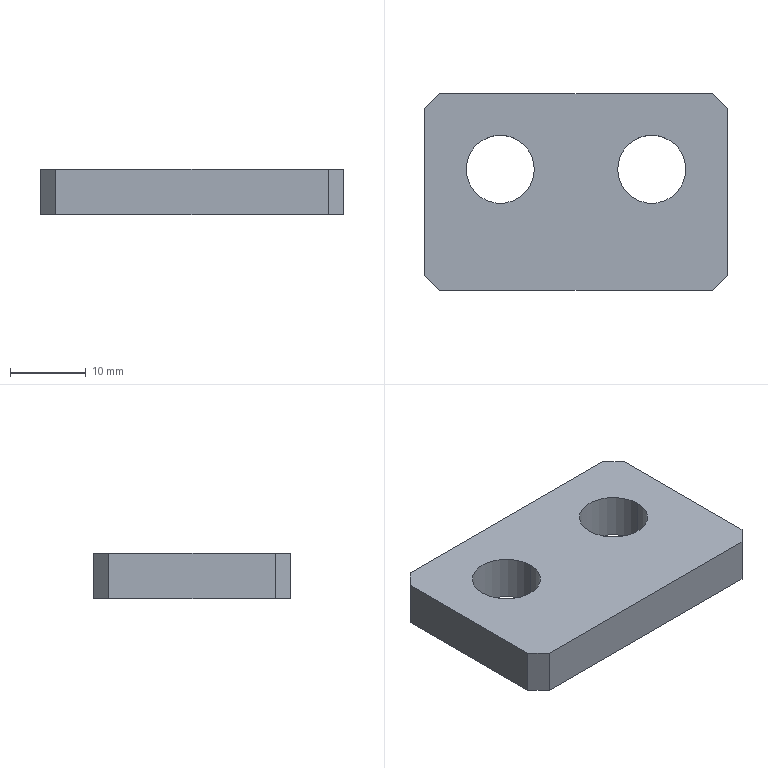Part | STEP file | 1 solid | 14 faces | box 40 x 26 x 6 mm | volume 5429 mm3 | plane 10 | cylinder 4 | commonest cylinder face diameters 9 x4
STEP:
#1=CARTESIAN_POINT('',(0.,0.,0.));
#2=DIRECTION('',(0.,0.,1.));
#3=DIRECTION('',(1.,0.,0.));
#4=AXIS2_PLACEMENT_3D('',#1,#2,#3);
#5=CARTESIAN_POINT('',(14.5,3.,6.));
#6=VERTEX_POINT('',#5);
#7=CARTESIAN_POINT('',(5.5,3.,6.));
#8=VERTEX_POINT('',#7);
#9=CARTESIAN_POINT('',(10.,3.,6.));
#10=DIRECTION('',(0.,0.,-1.));
#11=DIRECTION('',(1.,0.,0.));
#12=AXIS2_PLACEMENT_3D('',#9,#10,#11);
#13=CIRCLE('',#12,4.5);
#14=CARTESIAN_POINT('',(0.,0.,6.));
#15=DIRECTION('',(0.,0.,1.));
#16=DIRECTION('',(1.,0.,0.));
#17=AXIS2_PLACEMENT_3D('',#14,#15,#16);
#18=PLANE('',#17);
#19=CARTESIAN_POINT('',(14.5,3.));
#20=CARTESIAN_POINT('',(14.5,-4.794));
#21=CARTESIAN_POINT('',(7.75,-0.8971));
#22=CARTESIAN_POINT('',(1.,3.));
#23=CARTESIAN_POINT('',(7.75,6.897));
#24=CARTESIAN_POINT('',(14.5,10.794));
#25=CARTESIAN_POINT('',(14.5,3.));
#26=(BOUNDED_CURVE()B_SPLINE_CURVE(2,(#19,#20,#21,#22,#23,#24,#25),.UNSPECIFIED.,.T.,.F.)B_SPLINE_CURVE_WITH_KNOTS((1,2,2,2,2,1),(-2.094,0.,2.094,4.189,6.283,8.378),.UNSPECIFIED.)CURVE()GEOMETRIC_REPRESENTATION_ITEM()RATIONAL_B_SPLINE_CURVE((1.,0.5,1.,0.5,1.,0.5,1.))REPRESENTATION_ITEM(''));
#27=(GEOMETRIC_REPRESENTATION_CONTEXT(2)PARAMETRIC_REPRESENTATION_CONTEXT()REPRESENTATION_CONTEXT('',''));
#28=DEFINITIONAL_REPRESENTATION('',(#26),#27);
#29=PCURVE('',#18,#28);
#30=CARTESIAN_POINT('',(10.,3.,-0.001));
#31=DIRECTION('',(0.,0.,1.));
#32=DIRECTION('',(1.,0.,0.));
#33=AXIS2_PLACEMENT_3D('',#30,#31,#32);
#34=CYLINDRICAL_SURFACE('',#33,4.5);
#35=CARTESIAN_POINT('',(6.283,6.001));
#36=DIRECTION('',(-1.,0.));
#37=VECTOR('',#36,1.);
#38=LINE('',#35,#37);
#39=(GEOMETRIC_REPRESENTATION_CONTEXT(2)PARAMETRIC_REPRESENTATION_CONTEXT()REPRESENTATION_CONTEXT('',''));
#40=DEFINITIONAL_REPRESENTATION('',(#38),#39);
#41=PCURVE('',#34,#40);
#42=SURFACE_CURVE('',#13,(#29,#41),.PCURVE_S1.);
#43=EDGE_CURVE('',#6,#8,#42,.T.);
#44=ORIENTED_EDGE('',*,*,#43,.T.);
#45=CARTESIAN_POINT('',(10.,3.,6.));
#46=DIRECTION('',(0.,0.,-1.));
#47=DIRECTION('',(1.,0.,0.));
#48=AXIS2_PLACEMENT_3D('',#45,#46,#47);
#49=CIRCLE('',#48,4.5);
#50=CARTESIAN_POINT('',(14.5,3.));
#51=CARTESIAN_POINT('',(14.5,-4.794));
#52=CARTESIAN_POINT('',(7.75,-0.8971));
#53=CARTESIAN_POINT('',(1.,3.));
#54=CARTESIAN_POINT('',(7.75,6.897));
#55=CARTESIAN_POINT('',(14.5,10.794));
#56=CARTESIAN_POINT('',(14.5,3.));
#57=(BOUNDED_CURVE()B_SPLINE_CURVE(2,(#50,#51,#52,#53,#54,#55,#56),.UNSPECIFIED.,.T.,.F.)B_SPLINE_CURVE_WITH_KNOTS((1,2,2,2,2,1),(-2.094,0.,2.094,4.189,6.283,8.378),.UNSPECIFIED.)CURVE()GEOMETRIC_REPRESENTATION_ITEM()RATIONAL_B_SPLINE_CURVE((1.,0.5,1.,0.5,1.,0.5,1.))REPRESENTATION_ITEM(''));
#58=(GEOMETRIC_REPRESENTATION_CONTEXT(2)PARAMETRIC_REPRESENTATION_CONTEXT()REPRESENTATION_CONTEXT('',''));
#59=DEFINITIONAL_REPRESENTATION('',(#57),#58);
#60=PCURVE('',#18,#59);
#61=CARTESIAN_POINT('',(10.,3.,-0.001));
#62=DIRECTION('',(0.,0.,1.));
#63=DIRECTION('',(1.,0.,0.));
#64=AXIS2_PLACEMENT_3D('',#61,#62,#63);
#65=CYLINDRICAL_SURFACE('',#64,4.5);
#66=CARTESIAN_POINT('',(6.283,6.001));
#67=DIRECTION('',(-1.,0.));
#68=VECTOR('',#67,1.);
#69=LINE('',#66,#68);
#70=(GEOMETRIC_REPRESENTATION_CONTEXT(2)PARAMETRIC_REPRESENTATION_CONTEXT()REPRESENTATION_CONTEXT('',''));
#71=DEFINITIONAL_REPRESENTATION('',(#69),#70);
#72=PCURVE('',#65,#71);
#73=SURFACE_CURVE('',#49,(#60,#72),.PCURVE_S1.);
#74=EDGE_CURVE('',#8,#6,#73,.T.);
#75=ORIENTED_EDGE('',*,*,#74,.T.);
#76=EDGE_LOOP('',(#44,#75));
#77=FACE_BOUND('',#76,.T.);
#78=CARTESIAN_POINT('',(-5.5,3.,6.));
#79=VERTEX_POINT('',#78);
#80=CARTESIAN_POINT('',(-14.5,3.,6.));
#81=VERTEX_POINT('',#80);
#82=CARTESIAN_POINT('',(-10.,3.,6.));
#83=DIRECTION('',(0.,0.,-1.));
#84=DIRECTION('',(1.,0.,0.));
#85=AXIS2_PLACEMENT_3D('',#82,#83,#84);
#86=CIRCLE('',#85,4.5);
#87=CARTESIAN_POINT('',(-5.5,3.));
#88=CARTESIAN_POINT('',(-5.5,-4.794));
#89=CARTESIAN_POINT('',(-12.25,-0.8971));
#90=CARTESIAN_POINT('',(-19.,3.));
#91=CARTESIAN_POINT('',(-12.25,6.897));
#92=CARTESIAN_POINT('',(-5.5,10.794));
#93=CARTESIAN_POINT('',(-5.5,3.));
#94=(BOUNDED_CURVE()B_SPLINE_CURVE(2,(#87,#88,#89,#90,#91,#92,#93),.UNSPECIFIED.,.T.,.F.)B_SPLINE_CURVE_WITH_KNOTS((1,2,2,2,2,1),(-2.094,0.,2.094,4.189,6.283,8.378),.UNSPECIFIED.)CURVE()GEOMETRIC_REPRESENTATION_ITEM()RATIONAL_B_SPLINE_CURVE((1.,0.5,1.,0.5,1.,0.5,1.))REPRESENTATION_ITEM(''));
#95=(GEOMETRIC_REPRESENTATION_CONTEXT(2)PARAMETRIC_REPRESENTATION_CONTEXT()REPRESENTATION_CONTEXT('',''));
#96=DEFINITIONAL_REPRESENTATION('',(#94),#95);
#97=PCURVE('',#18,#96);
#98=CARTESIAN_POINT('',(-10.,3.,-0.001));
#99=DIRECTION('',(0.,0.,1.));
#100=DIRECTION('',(1.,0.,0.));
#101=AXIS2_PLACEMENT_3D('',#98,#99,#100);
#102=CYLINDRICAL_SURFACE('',#101,4.5);
#103=CARTESIAN_POINT('',(6.283,6.001));
#104=DIRECTION('',(-1.,0.));
#105=VECTOR('',#104,1.);
#106=LINE('',#103,#105);
#107=(GEOMETRIC_REPRESENTATION_CONTEXT(2)PARAMETRIC_REPRESENTATION_CONTEXT()REPRESENTATION_CONTEXT('',''));
#108=DEFINITIONAL_REPRESENTATION('',(#106),#107);
#109=PCURVE('',#102,#108);
#110=SURFACE_CURVE('',#86,(#97,#109),.PCURVE_S1.);
#111=EDGE_CURVE('',#79,#81,#110,.T.);
#112=ORIENTED_EDGE('',*,*,#111,.T.);
#113=CARTESIAN_POINT('',(-10.,3.,6.));
#114=DIRECTION('',(0.,0.,-1.));
#115=DIRECTION('',(1.,0.,0.));
#116=AXIS2_PLACEMENT_3D('',#113,#114,#115);
#117=CIRCLE('',#116,4.5);
#118=CARTESIAN_POINT('',(-5.5,3.));
#119=CARTESIAN_POINT('',(-5.5,-4.794));
#120=CARTESIAN_POINT('',(-12.25,-0.8971));
#121=CARTESIAN_POINT('',(-19.,3.));
#122=CARTESIAN_POINT('',(-12.25,6.897));
#123=CARTESIAN_POINT('',(-5.5,10.794));
#124=CARTESIAN_POINT('',(-5.5,3.));
#125=(BOUNDED_CURVE()B_SPLINE_CURVE(2,(#118,#119,#120,#121,#122,#123,#124),.UNSPECIFIED.,.T.,.F.)B_SPLINE_CURVE_WITH_KNOTS((1,2,2,2,2,1),(-2.094,0.,2.094,4.189,6.283,8.378),.UNSPECIFIED.)CURVE()GEOMETRIC_REPRESENTATION_ITEM()RATIONAL_B_SPLINE_CURVE((1.,0.5,1.,0.5,1.,0.5,1.))REPRESENTATION_ITEM(''));
#126=(GEOMETRIC_REPRESENTATION_CONTEXT(2)PARAMETRIC_REPRESENTATION_CONTEXT()REPRESENTATION_CONTEXT('',''));
#127=DEFINITIONAL_REPRESENTATION('',(#125),#126);
#128=PCURVE('',#18,#127);
#129=CARTESIAN_POINT('',(-10.,3.,-0.001));
#130=DIRECTION('',(0.,0.,1.));
#131=DIRECTION('',(1.,0.,0.));
#132=AXIS2_PLACEMENT_3D('',#129,#130,#131);
#133=CYLINDRICAL_SURFACE('',#132,4.5);
#134=CARTESIAN_POINT('',(6.283,6.001));
#135=DIRECTION('',(-1.,0.));
#136=VECTOR('',#135,1.);
#137=LINE('',#134,#136);
#138=(GEOMETRIC_REPRESENTATION_CONTEXT(2)PARAMETRIC_REPRESENTATION_CONTEXT()REPRESENTATION_CONTEXT('',''));
#139=DEFINITIONAL_REPRESENTATION('',(#137),#138);
#140=PCURVE('',#133,#139);
#141=SURFACE_CURVE('',#117,(#128,#140),.PCURVE_S1.);
#142=EDGE_CURVE('',#81,#79,#141,.T.);
#143=ORIENTED_EDGE('',*,*,#142,.T.);
#144=EDGE_LOOP('',(#112,#143));
#145=FACE_BOUND('',#144,.T.);
#146=CARTESIAN_POINT('',(18.,13.,6.));
#147=VERTEX_POINT('',#146);
#148=CARTESIAN_POINT('',(-18.,13.,6.));
#149=VERTEX_POINT('',#148);
#150=CARTESIAN_POINT('',(20.,13.,6.));
#151=DIRECTION('',(-1.,0.,0.));
#152=VECTOR('',#151,1.);
#153=LINE('',#150,#152);
#154=CARTESIAN_POINT('',(20.,13.));
#155=DIRECTION('',(-1.,0.));
#156=VECTOR('',#155,1.);
#157=LINE('',#154,#156);
#158=(GEOMETRIC_REPRESENTATION_CONTEXT(2)PARAMETRIC_REPRESENTATION_CONTEXT()REPRESENTATION_CONTEXT('',''));
#159=DEFINITIONAL_REPRESENTATION('',(#157),#158);
#160=PCURVE('',#18,#159);
#161=CARTESIAN_POINT('',(20.,13.,6.));
#162=DIRECTION('',(0.,-1.,0.));
#163=DIRECTION('',(0.,0.,-1.));
#164=AXIS2_PLACEMENT_3D('',#161,#162,#163);
#165=PLANE('',#164);
#166=CARTESIAN_POINT('',(0.,0.));
#167=DIRECTION('',(0.,-1.));
#168=VECTOR('',#167,1.);
#169=LINE('',#166,#168);
#170=(GEOMETRIC_REPRESENTATION_CONTEXT(2)PARAMETRIC_REPRESENTATION_CONTEXT()REPRESENTATION_CONTEXT('',''));
#171=DEFINITIONAL_REPRESENTATION('',(#169),#170);
#172=PCURVE('',#165,#171);
#173=SURFACE_CURVE('',#153,(#160,#172),.PCURVE_S1.);
#174=EDGE_CURVE('',#147,#149,#173,.T.);
#175=ORIENTED_EDGE('',*,*,#174,.T.);
#176=CARTESIAN_POINT('',(-20.,11.,6.));
#177=VERTEX_POINT('',#176);
#178=CARTESIAN_POINT('',(-20.,11.,6.));
#179=DIRECTION('',(-0.7071,-0.7071,0.));
#180=VECTOR('',#179,1.);
#181=LINE('',#178,#180);
#182=CARTESIAN_POINT('',(-20.,11.));
#183=DIRECTION('',(-0.7071,-0.7071));
#184=VECTOR('',#183,1.);
#185=LINE('',#182,#184);
#186=(GEOMETRIC_REPRESENTATION_CONTEXT(2)PARAMETRIC_REPRESENTATION_CONTEXT()REPRESENTATION_CONTEXT('',''));
#187=DEFINITIONAL_REPRESENTATION('',(#185),#186);
#188=PCURVE('',#18,#187);
#189=CARTESIAN_POINT('',(-20.,11.,6.));
#190=DIRECTION('',(0.7071,-0.7071,0.));
#191=DIRECTION('',(0.,0.,-1.));
#192=AXIS2_PLACEMENT_3D('',#189,#190,#191);
#193=PLANE('',#192);
#194=CARTESIAN_POINT('',(0.,0.));
#195=DIRECTION('',(0.,-1.));
#196=VECTOR('',#195,1.);
#197=LINE('',#194,#196);
#198=(GEOMETRIC_REPRESENTATION_CONTEXT(2)PARAMETRIC_REPRESENTATION_CONTEXT()REPRESENTATION_CONTEXT('',''));
#199=DEFINITIONAL_REPRESENTATION('',(#197),#198);
#200=PCURVE('',#193,#199);
#201=SURFACE_CURVE('',#181,(#188,#200),.PCURVE_S1.);
#202=EDGE_CURVE('',#149,#177,#201,.T.);
#203=ORIENTED_EDGE('',*,*,#202,.T.);
#204=CARTESIAN_POINT('',(-20.,-11.,6.));
#205=VERTEX_POINT('',#204);
#206=CARTESIAN_POINT('',(-20.,-13.,6.));
#207=DIRECTION('',(0.,-1.,0.));
#208=VECTOR('',#207,1.);
#209=LINE('',#206,#208);
#210=CARTESIAN_POINT('',(-20.,-13.));
#211=DIRECTION('',(0.,-1.));
#212=VECTOR('',#211,1.);
#213=LINE('',#210,#212);
#214=(GEOMETRIC_REPRESENTATION_CONTEXT(2)PARAMETRIC_REPRESENTATION_CONTEXT()REPRESENTATION_CONTEXT('',''));
#215=DEFINITIONAL_REPRESENTATION('',(#213),#214);
#216=PCURVE('',#18,#215);
#217=CARTESIAN_POINT('',(-20.,-13.,6.));
#218=DIRECTION('',(1.,0.,0.));
#219=DIRECTION('',(0.,1.,0.));
#220=AXIS2_PLACEMENT_3D('',#217,#218,#219);
#221=PLANE('',#220);
#222=CARTESIAN_POINT('',(0.,0.));
#223=DIRECTION('',(-1.,0.));
#224=VECTOR('',#223,1.);
#225=LINE('',#222,#224);
#226=(GEOMETRIC_REPRESENTATION_CONTEXT(2)PARAMETRIC_REPRESENTATION_CONTEXT()REPRESENTATION_CONTEXT('',''));
#227=DEFINITIONAL_REPRESENTATION('',(#225),#226);
#228=PCURVE('',#221,#227);
#229=SURFACE_CURVE('',#209,(#216,#228),.PCURVE_S1.);
#230=EDGE_CURVE('',#177,#205,#229,.T.);
#231=ORIENTED_EDGE('',*,*,#230,.T.);
#232=CARTESIAN_POINT('',(-18.,-13.,6.));
#233=VERTEX_POINT('',#232);
#234=CARTESIAN_POINT('',(-18.,-13.,6.));
#235=DIRECTION('',(0.7071,-0.7071,0.));
#236=VECTOR('',#235,1.);
#237=LINE('',#234,#236);
#238=CARTESIAN_POINT('',(-18.,-13.));
#239=DIRECTION('',(0.7071,-0.7071));
#240=VECTOR('',#239,1.);
#241=LINE('',#238,#240);
#242=(GEOMETRIC_REPRESENTATION_CONTEXT(2)PARAMETRIC_REPRESENTATION_CONTEXT()REPRESENTATION_CONTEXT('',''));
#243=DEFINITIONAL_REPRESENTATION('',(#241),#242);
#244=PCURVE('',#18,#243);
#245=CARTESIAN_POINT('',(-18.,-13.,6.));
#246=DIRECTION('',(0.7071,0.7071,0.));
#247=DIRECTION('',(0.,0.,-1.));
#248=AXIS2_PLACEMENT_3D('',#245,#246,#247);
#249=PLANE('',#248);
#250=CARTESIAN_POINT('',(0.,0.));
#251=DIRECTION('',(0.,-1.));
#252=VECTOR('',#251,1.);
#253=LINE('',#250,#252);
#254=(GEOMETRIC_REPRESENTATION_CONTEXT(2)PARAMETRIC_REPRESENTATION_CONTEXT()REPRESENTATION_CONTEXT('',''));
#255=DEFINITIONAL_REPRESENTATION('',(#253),#254);
#256=PCURVE('',#249,#255);
#257=SURFACE_CURVE('',#237,(#244,#256),.PCURVE_S1.);
#258=EDGE_CURVE('',#205,#233,#257,.T.);
#259=ORIENTED_EDGE('',*,*,#258,.T.);
#260=CARTESIAN_POINT('',(18.,-13.,6.));
#261=VERTEX_POINT('',#260);
#262=CARTESIAN_POINT('',(20.,-13.,6.));
#263=DIRECTION('',(1.,0.,0.));
#264=VECTOR('',#263,1.);
#265=LINE('',#262,#264);
#266=CARTESIAN_POINT('',(20.,-13.));
#267=DIRECTION('',(1.,0.));
#268=VECTOR('',#267,1.);
#269=LINE('',#266,#268);
#270=(GEOMETRIC_REPRESENTATION_CONTEXT(2)PARAMETRIC_REPRESENTATION_CONTEXT()REPRESENTATION_CONTEXT('',''));
#271=DEFINITIONAL_REPRESENTATION('',(#269),#270);
#272=PCURVE('',#18,#271);
#273=CARTESIAN_POINT('',(20.,-13.,6.));
#274=DIRECTION('',(0.,1.,0.));
#275=DIRECTION('',(1.,0.,0.));
#276=AXIS2_PLACEMENT_3D('',#273,#274,#275);
#277=PLANE('',#276);
#278=CARTESIAN_POINT('',(0.,0.));
#279=DIRECTION('',(1.,0.));
#280=VECTOR('',#279,1.);
#281=LINE('',#278,#280);
#282=(GEOMETRIC_REPRESENTATION_CONTEXT(2)PARAMETRIC_REPRESENTATION_CONTEXT()REPRESENTATION_CONTEXT('',''));
#283=DEFINITIONAL_REPRESENTATION('',(#281),#282);
#284=PCURVE('',#277,#283);
#285=SURFACE_CURVE('',#265,(#272,#284),.PCURVE_S1.);
#286=EDGE_CURVE('',#233,#261,#285,.T.);
#287=ORIENTED_EDGE('',*,*,#286,.T.);
#288=CARTESIAN_POINT('',(20.,-11.,6.));
#289=VERTEX_POINT('',#288);
#290=CARTESIAN_POINT('',(20.,-11.,6.));
#291=DIRECTION('',(0.7071,0.7071,0.));
#292=VECTOR('',#291,1.);
#293=LINE('',#290,#292);
#294=CARTESIAN_POINT('',(20.,-11.));
#295=DIRECTION('',(0.7071,0.7071));
#296=VECTOR('',#295,1.);
#297=LINE('',#294,#296);
#298=(GEOMETRIC_REPRESENTATION_CONTEXT(2)PARAMETRIC_REPRESENTATION_CONTEXT()REPRESENTATION_CONTEXT('',''));
#299=DEFINITIONAL_REPRESENTATION('',(#297),#298);
#300=PCURVE('',#18,#299);
#301=CARTESIAN_POINT('',(20.,-11.,6.));
#302=DIRECTION('',(-0.7071,0.7071,0.));
#303=DIRECTION('',(0.,0.,1.));
#304=AXIS2_PLACEMENT_3D('',#301,#302,#303);
#305=PLANE('',#304);
#306=CARTESIAN_POINT('',(0.,0.));
#307=DIRECTION('',(0.,1.));
#308=VECTOR('',#307,1.);
#309=LINE('',#306,#308);
#310=(GEOMETRIC_REPRESENTATION_CONTEXT(2)PARAMETRIC_REPRESENTATION_CONTEXT()REPRESENTATION_CONTEXT('',''));
#311=DEFINITIONAL_REPRESENTATION('',(#309),#310);
#312=PCURVE('',#305,#311);
#313=SURFACE_CURVE('',#293,(#300,#312),.PCURVE_S1.);
#314=EDGE_CURVE('',#261,#289,#313,.T.);
#315=ORIENTED_EDGE('',*,*,#314,.T.);
#316=CARTESIAN_POINT('',(20.,11.,6.));
#317=VERTEX_POINT('',#316);
#318=CARTESIAN_POINT('',(20.,-13.,6.));
#319=DIRECTION('',(0.,1.,0.));
#320=VECTOR('',#319,1.);
#321=LINE('',#318,#320);
#322=CARTESIAN_POINT('',(20.,-13.));
#323=DIRECTION('',(0.,1.));
#324=VECTOR('',#323,1.);
#325=LINE('',#322,#324);
#326=(GEOMETRIC_REPRESENTATION_CONTEXT(2)PARAMETRIC_REPRESENTATION_CONTEXT()REPRESENTATION_CONTEXT('',''));
#327=DEFINITIONAL_REPRESENTATION('',(#325),#326);
#328=PCURVE('',#18,#327);
#329=CARTESIAN_POINT('',(20.,-13.,6.));
#330=DIRECTION('',(-1.,0.,0.));
#331=DIRECTION('',(0.,0.,1.));
#332=AXIS2_PLACEMENT_3D('',#329,#330,#331);
#333=PLANE('',#332);
#334=CARTESIAN_POINT('',(0.,0.));
#335=DIRECTION('',(0.,1.));
#336=VECTOR('',#335,1.);
#337=LINE('',#334,#336);
#338=(GEOMETRIC_REPRESENTATION_CONTEXT(2)PARAMETRIC_REPRESENTATION_CONTEXT()REPRESENTATION_CONTEXT('',''));
#339=DEFINITIONAL_REPRESENTATION('',(#337),#338);
#340=PCURVE('',#333,#339);
#341=SURFACE_CURVE('',#321,(#328,#340),.PCURVE_S1.);
#342=EDGE_CURVE('',#289,#317,#341,.T.);
#343=ORIENTED_EDGE('',*,*,#342,.T.);
#344=CARTESIAN_POINT('',(18.,13.,6.));
#345=DIRECTION('',(-0.7071,0.7071,0.));
#346=VECTOR('',#345,1.);
#347=LINE('',#344,#346);
#348=CARTESIAN_POINT('',(18.,13.));
#349=DIRECTION('',(-0.7071,0.7071));
#350=VECTOR('',#349,1.);
#351=LINE('',#348,#350);
#352=(GEOMETRIC_REPRESENTATION_CONTEXT(2)PARAMETRIC_REPRESENTATION_CONTEXT()REPRESENTATION_CONTEXT('',''));
#353=DEFINITIONAL_REPRESENTATION('',(#351),#352);
#354=PCURVE('',#18,#353);
#355=CARTESIAN_POINT('',(18.,13.,6.));
#356=DIRECTION('',(-0.7071,-0.7071,0.));
#357=DIRECTION('',(-0.7071,0.7071,0.));
#358=AXIS2_PLACEMENT_3D('',#355,#356,#357);
#359=PLANE('',#358);
#360=CARTESIAN_POINT('',(0.,0.));
#361=DIRECTION('',(1.,0.));
#362=VECTOR('',#361,1.);
#363=LINE('',#360,#362);
#364=(GEOMETRIC_REPRESENTATION_CONTEXT(2)PARAMETRIC_REPRESENTATION_CONTEXT()REPRESENTATION_CONTEXT('',''));
#365=DEFINITIONAL_REPRESENTATION('',(#363),#364);
#366=PCURVE('',#359,#365);
#367=SURFACE_CURVE('',#347,(#354,#366),.PCURVE_S1.);
#368=EDGE_CURVE('',#317,#147,#367,.T.);
#369=ORIENTED_EDGE('',*,*,#368,.T.);
#370=EDGE_LOOP('',(#175,#203,#231,#259,#287,#315,#343,#369));
#371=FACE_BOUND('',#370,.T.);
#372=ADVANCED_FACE('',(#77,#145,#371),#18,.T.);
#373=ORIENTED_EDGE('',*,*,#74,.T.);
#374=CARTESIAN_POINT('',(14.5,3.,0.));
#375=VERTEX_POINT('',#374);
#376=CARTESIAN_POINT('',(14.5,3.,-0.001));
#377=DIRECTION('',(0.,0.,1.));
#378=VECTOR('',#377,1.);
#379=LINE('',#376,#378);
#380=CARTESIAN_POINT('',(0.,0.));
#381=DIRECTION('',(0.,1.));
#382=VECTOR('',#381,1.);
#383=LINE('',#380,#382);
#384=(GEOMETRIC_REPRESENTATION_CONTEXT(2)PARAMETRIC_REPRESENTATION_CONTEXT()REPRESENTATION_CONTEXT('',''));
#385=DEFINITIONAL_REPRESENTATION('',(#383),#384);
#386=PCURVE('',#65,#385);
#387=CARTESIAN_POINT('',(6.283,0.));
#388=DIRECTION('',(0.,1.));
#389=VECTOR('',#388,1.);
#390=LINE('',#387,#389);
#391=(GEOMETRIC_REPRESENTATION_CONTEXT(2)PARAMETRIC_REPRESENTATION_CONTEXT()REPRESENTATION_CONTEXT('',''));
#392=DEFINITIONAL_REPRESENTATION('',(#390),#391);
#393=PCURVE('',#34,#392);
#394=SURFACE_CURVE('',#379,(#386,#393),.PCURVE_S1.);
#395=EDGE_CURVE('',#375,#6,#394,.T.);
#396=ORIENTED_EDGE('',*,*,#395,.F.);
#397=CARTESIAN_POINT('',(5.5,3.,0.));
#398=VERTEX_POINT('',#397);
#399=CARTESIAN_POINT('',(10.,3.,0.));
#400=DIRECTION('',(0.,0.,-1.));
#401=DIRECTION('',(1.,0.,0.));
#402=AXIS2_PLACEMENT_3D('',#399,#400,#401);
#403=CIRCLE('',#402,4.5);
#404=CARTESIAN_POINT('',(6.283,0.001));
#405=DIRECTION('',(-1.,0.));
#406=VECTOR('',#405,1.);
#407=LINE('',#404,#406);
#408=(GEOMETRIC_REPRESENTATION_CONTEXT(2)PARAMETRIC_REPRESENTATION_CONTEXT()REPRESENTATION_CONTEXT('',''));
#409=DEFINITIONAL_REPRESENTATION('',(#407),#408);
#410=PCURVE('',#65,#409);
#411=CARTESIAN_POINT('',(0.,0.,0.));
#412=DIRECTION('',(0.,0.,1.));
#413=DIRECTION('',(1.,0.,0.));
#414=AXIS2_PLACEMENT_3D('',#411,#412,#413);
#415=PLANE('',#414);
#416=CARTESIAN_POINT('',(14.5,3.));
#417=CARTESIAN_POINT('',(14.5,-4.794));
#418=CARTESIAN_POINT('',(7.75,-0.8971));
#419=CARTESIAN_POINT('',(1.,3.));
#420=CARTESIAN_POINT('',(7.75,6.897));
#421=CARTESIAN_POINT('',(14.5,10.794));
#422=CARTESIAN_POINT('',(14.5,3.));
#423=(BOUNDED_CURVE()B_SPLINE_CURVE(2,(#416,#417,#418,#419,#420,#421,#422),.UNSPECIFIED.,.T.,.F.)B_SPLINE_CURVE_WITH_KNOTS((1,2,2,2,2,1),(-2.094,0.,2.094,4.189,6.283,8.378),.UNSPECIFIED.)CURVE()GEOMETRIC_REPRESENTATION_ITEM()RATIONAL_B_SPLINE_CURVE((1.,0.5,1.,0.5,1.,0.5,1.))REPRESENTATION_ITEM(''));
#424=(GEOMETRIC_REPRESENTATION_CONTEXT(2)PARAMETRIC_REPRESENTATION_CONTEXT()REPRESENTATION_CONTEXT('',''));
#425=DEFINITIONAL_REPRESENTATION('',(#423),#424);
#426=PCURVE('',#415,#425);
#427=SURFACE_CURVE('',#403,(#410,#426),.PCURVE_S1.);
#428=EDGE_CURVE('',#398,#375,#427,.T.);
#429=ORIENTED_EDGE('',*,*,#428,.F.);
#430=CARTESIAN_POINT('',(5.5,3.,-0.001));
#431=DIRECTION('',(0.,0.,1.));
#432=VECTOR('',#431,1.);
#433=LINE('',#430,#432);
#434=CARTESIAN_POINT('',(3.142,0.));
#435=DIRECTION('',(0.,1.));
#436=VECTOR('',#435,1.);
#437=LINE('',#434,#436);
#438=(GEOMETRIC_REPRESENTATION_CONTEXT(2)PARAMETRIC_REPRESENTATION_CONTEXT()REPRESENTATION_CONTEXT('',''));
#439=DEFINITIONAL_REPRESENTATION('',(#437),#438);
#440=PCURVE('',#65,#439);
#441=CARTESIAN_POINT('',(3.142,0.));
#442=DIRECTION('',(0.,1.));
#443=VECTOR('',#442,1.);
#444=LINE('',#441,#443);
#445=(GEOMETRIC_REPRESENTATION_CONTEXT(2)PARAMETRIC_REPRESENTATION_CONTEXT()REPRESENTATION_CONTEXT('',''));
#446=DEFINITIONAL_REPRESENTATION('',(#444),#445);
#447=PCURVE('',#34,#446);
#448=SURFACE_CURVE('',#433,(#440,#447),.PCURVE_S1.);
#449=EDGE_CURVE('',#398,#8,#448,.T.);
#450=ORIENTED_EDGE('',*,*,#449,.T.);
#451=EDGE_LOOP('',(#373,#396,#429,#450));
#452=FACE_BOUND('',#451,.F.);
#453=ADVANCED_FACE('',(#452),#65,.F.);
#454=ORIENTED_EDGE('',*,*,#142,.T.);
#455=CARTESIAN_POINT('',(-5.5,3.,0.));
#456=VERTEX_POINT('',#455);
#457=CARTESIAN_POINT('',(-5.5,3.,-0.001));
#458=DIRECTION('',(0.,0.,1.));
#459=VECTOR('',#458,1.);
#460=LINE('',#457,#459);
#461=CARTESIAN_POINT('',(0.,0.));
#462=DIRECTION('',(0.,1.));
#463=VECTOR('',#462,1.);
#464=LINE('',#461,#463);
#465=(GEOMETRIC_REPRESENTATION_CONTEXT(2)PARAMETRIC_REPRESENTATION_CONTEXT()REPRESENTATION_CONTEXT('',''));
#466=DEFINITIONAL_REPRESENTATION('',(#464),#465);
#467=PCURVE('',#133,#466);
#468=CARTESIAN_POINT('',(6.283,0.));
#469=DIRECTION('',(0.,1.));
#470=VECTOR('',#469,1.);
#471=LINE('',#468,#470);
#472=(GEOMETRIC_REPRESENTATION_CONTEXT(2)PARAMETRIC_REPRESENTATION_CONTEXT()REPRESENTATION_CONTEXT('',''));
#473=DEFINITIONAL_REPRESENTATION('',(#471),#472);
#474=PCURVE('',#102,#473);
#475=SURFACE_CURVE('',#460,(#467,#474),.PCURVE_S1.);
#476=EDGE_CURVE('',#456,#79,#475,.T.);
#477=ORIENTED_EDGE('',*,*,#476,.F.);
#478=CARTESIAN_POINT('',(-14.5,3.,0.));
#479=VERTEX_POINT('',#478);
#480=CARTESIAN_POINT('',(-10.,3.,0.));
#481=DIRECTION('',(0.,0.,-1.));
#482=DIRECTION('',(1.,0.,0.));
#483=AXIS2_PLACEMENT_3D('',#480,#481,#482);
#484=CIRCLE('',#483,4.5);
#485=CARTESIAN_POINT('',(6.283,0.001));
#486=DIRECTION('',(-1.,0.));
#487=VECTOR('',#486,1.);
#488=LINE('',#485,#487);
#489=(GEOMETRIC_REPRESENTATION_CONTEXT(2)PARAMETRIC_REPRESENTATION_CONTEXT()REPRESENTATION_CONTEXT('',''));
#490=DEFINITIONAL_REPRESENTATION('',(#488),#489);
#491=PCURVE('',#133,#490);
#492=CARTESIAN_POINT('',(-5.5,3.));
#493=CARTESIAN_POINT('',(-5.5,-4.794));
#494=CARTESIAN_POINT('',(-12.25,-0.8971));
#495=CARTESIAN_POINT('',(-19.,3.));
#496=CARTESIAN_POINT('',(-12.25,6.897));
#497=CARTESIAN_POINT('',(-5.5,10.794));
#498=CARTESIAN_POINT('',(-5.5,3.));
#499=(BOUNDED_CURVE()B_SPLINE_CURVE(2,(#492,#493,#494,#495,#496,#497,#498),.UNSPECIFIED.,.T.,.F.)B_SPLINE_CURVE_WITH_KNOTS((1,2,2,2,2,1),(-2.094,0.,2.094,4.189,6.283,8.378),.UNSPECIFIED.)CURVE()GEOMETRIC_REPRESENTATION_ITEM()RATIONAL_B_SPLINE_CURVE((1.,0.5,1.,0.5,1.,0.5,1.))REPRESENTATION_ITEM(''));
#500=(GEOMETRIC_REPRESENTATION_CONTEXT(2)PARAMETRIC_REPRESENTATION_CONTEXT()REPRESENTATION_CONTEXT('',''));
#501=DEFINITIONAL_REPRESENTATION('',(#499),#500);
#502=PCURVE('',#415,#501);
#503=SURFACE_CURVE('',#484,(#491,#502),.PCURVE_S1.);
#504=EDGE_CURVE('',#479,#456,#503,.T.);
#505=ORIENTED_EDGE('',*,*,#504,.F.);
#506=CARTESIAN_POINT('',(-14.5,3.,-0.001));
#507=DIRECTION('',(0.,0.,1.));
#508=VECTOR('',#507,1.);
#509=LINE('',#506,#508);
#510=CARTESIAN_POINT('',(3.142,0.));
#511=DIRECTION('',(0.,1.));
#512=VECTOR('',#511,1.);
#513=LINE('',#510,#512);
#514=(GEOMETRIC_REPRESENTATION_CONTEXT(2)PARAMETRIC_REPRESENTATION_CONTEXT()REPRESENTATION_CONTEXT('',''));
#515=DEFINITIONAL_REPRESENTATION('',(#513),#514);
#516=PCURVE('',#133,#515);
#517=CARTESIAN_POINT('',(3.142,0.));
#518=DIRECTION('',(0.,1.));
#519=VECTOR('',#518,1.);
#520=LINE('',#517,#519);
#521=(GEOMETRIC_REPRESENTATION_CONTEXT(2)PARAMETRIC_REPRESENTATION_CONTEXT()REPRESENTATION_CONTEXT('',''));
#522=DEFINITIONAL_REPRESENTATION('',(#520),#521);
#523=PCURVE('',#102,#522);
#524=SURFACE_CURVE('',#509,(#516,#523),.PCURVE_S1.);
#525=EDGE_CURVE('',#479,#81,#524,.T.);
#526=ORIENTED_EDGE('',*,*,#525,.T.);
#527=EDGE_LOOP('',(#454,#477,#505,#526));
#528=FACE_BOUND('',#527,.F.);
#529=ADVANCED_FACE('',(#528),#133,.F.);
#530=CARTESIAN_POINT('',(18.,-13.,0.));
#531=VERTEX_POINT('',#530);
#532=CARTESIAN_POINT('',(18.,-13.,6.));
#533=DIRECTION('',(0.,0.,-1.));
#534=VECTOR('',#533,1.);
#535=LINE('',#532,#534);
#536=CARTESIAN_POINT('',(0.,-2.828));
#537=DIRECTION('',(-1.,0.));
#538=VECTOR('',#537,1.);
#539=LINE('',#536,#538);
#540=(GEOMETRIC_REPRESENTATION_CONTEXT(2)PARAMETRIC_REPRESENTATION_CONTEXT()REPRESENTATION_CONTEXT('',''));
#541=DEFINITIONAL_REPRESENTATION('',(#539),#540);
#542=PCURVE('',#305,#541);
#543=CARTESIAN_POINT('',(-2.,0.));
#544=DIRECTION('',(0.,1.));
#545=VECTOR('',#544,1.);
#546=LINE('',#543,#545);
#547=(GEOMETRIC_REPRESENTATION_CONTEXT(2)PARAMETRIC_REPRESENTATION_CONTEXT()REPRESENTATION_CONTEXT('',''));
#548=DEFINITIONAL_REPRESENTATION('',(#546),#547);
#549=PCURVE('',#277,#548);
#550=SURFACE_CURVE('',#535,(#542,#549),.PCURVE_S1.);
#551=EDGE_CURVE('',#261,#531,#550,.T.);
#552=ORIENTED_EDGE('',*,*,#551,.T.);
#553=CARTESIAN_POINT('',(20.,-11.,0.));
#554=VERTEX_POINT('',#553);
#555=CARTESIAN_POINT('',(18.,-13.,0.));
#556=DIRECTION('',(0.7071,0.7071,0.));
#557=VECTOR('',#556,1.);
#558=LINE('',#555,#557);
#559=CARTESIAN_POINT('',(-6.,-2.828));
#560=DIRECTION('',(0.,1.));
#561=VECTOR('',#560,1.);
#562=LINE('',#559,#561);
#563=(GEOMETRIC_REPRESENTATION_CONTEXT(2)PARAMETRIC_REPRESENTATION_CONTEXT()REPRESENTATION_CONTEXT('',''));
#564=DEFINITIONAL_REPRESENTATION('',(#562),#563);
#565=PCURVE('',#305,#564);
#566=CARTESIAN_POINT('',(18.,-13.));
#567=DIRECTION('',(0.7071,0.7071));
#568=VECTOR('',#567,1.);
#569=LINE('',#566,#568);
#570=(GEOMETRIC_REPRESENTATION_CONTEXT(2)PARAMETRIC_REPRESENTATION_CONTEXT()REPRESENTATION_CONTEXT('',''));
#571=DEFINITIONAL_REPRESENTATION('',(#569),#570);
#572=PCURVE('',#415,#571);
#573=SURFACE_CURVE('',#558,(#565,#572),.PCURVE_S1.);
#574=EDGE_CURVE('',#531,#554,#573,.T.);
#575=ORIENTED_EDGE('',*,*,#574,.T.);
#576=CARTESIAN_POINT('',(20.,-11.,6.));
#577=DIRECTION('',(0.,0.,1.));
#578=VECTOR('',#577,1.);
#579=LINE('',#576,#578);
#580=CARTESIAN_POINT('',(0.,0.));
#581=DIRECTION('',(1.,0.));
#582=VECTOR('',#581,1.);
#583=LINE('',#580,#582);
#584=(GEOMETRIC_REPRESENTATION_CONTEXT(2)PARAMETRIC_REPRESENTATION_CONTEXT()REPRESENTATION_CONTEXT('',''));
#585=DEFINITIONAL_REPRESENTATION('',(#583),#584);
#586=PCURVE('',#305,#585);
#587=CARTESIAN_POINT('',(0.,2.));
#588=DIRECTION('',(1.,0.));
#589=VECTOR('',#588,1.);
#590=LINE('',#587,#589);
#591=(GEOMETRIC_REPRESENTATION_CONTEXT(2)PARAMETRIC_REPRESENTATION_CONTEXT()REPRESENTATION_CONTEXT('',''));
#592=DEFINITIONAL_REPRESENTATION('',(#590),#591);
#593=PCURVE('',#333,#592);
#594=SURFACE_CURVE('',#579,(#586,#593),.PCURVE_S1.);
#595=EDGE_CURVE('',#554,#289,#594,.T.);
#596=ORIENTED_EDGE('',*,*,#595,.T.);
#597=ORIENTED_EDGE('',*,*,#314,.F.);
#598=EDGE_LOOP('',(#552,#575,#596,#597));
#599=FACE_BOUND('',#598,.T.);
#600=ADVANCED_FACE('',(#599),#305,.F.);
#601=ORIENTED_EDGE('',*,*,#595,.F.);
#602=CARTESIAN_POINT('',(20.,11.,0.));
#603=VERTEX_POINT('',#602);
#604=CARTESIAN_POINT('',(20.,0.,0.));
#605=DIRECTION('',(0.,1.,0.));
#606=VECTOR('',#605,1.);
#607=LINE('',#604,#606);
#608=CARTESIAN_POINT('',(-6.,13.));
#609=DIRECTION('',(0.,1.));
#610=VECTOR('',#609,1.);
#611=LINE('',#608,#610);
#612=(GEOMETRIC_REPRESENTATION_CONTEXT(2)PARAMETRIC_REPRESENTATION_CONTEXT()REPRESENTATION_CONTEXT('',''));
#613=DEFINITIONAL_REPRESENTATION('',(#611),#612);
#614=PCURVE('',#333,#613);
#615=CARTESIAN_POINT('',(20.,0.));
#616=DIRECTION('',(0.,1.));
#617=VECTOR('',#616,1.);
#618=LINE('',#615,#617);
#619=(GEOMETRIC_REPRESENTATION_CONTEXT(2)PARAMETRIC_REPRESENTATION_CONTEXT()REPRESENTATION_CONTEXT('',''));
#620=DEFINITIONAL_REPRESENTATION('',(#618),#619);
#621=PCURVE('',#415,#620);
#622=SURFACE_CURVE('',#607,(#614,#621),.PCURVE_S1.);
#623=EDGE_CURVE('',#554,#603,#622,.T.);
#624=ORIENTED_EDGE('',*,*,#623,.T.);
#625=CARTESIAN_POINT('',(20.,11.,6.));
#626=DIRECTION('',(0.,0.,1.));
#627=VECTOR('',#626,1.);
#628=LINE('',#625,#627);
#629=CARTESIAN_POINT('',(0.,24.));
#630=DIRECTION('',(1.,0.));
#631=VECTOR('',#630,1.);
#632=LINE('',#629,#631);
#633=(GEOMETRIC_REPRESENTATION_CONTEXT(2)PARAMETRIC_REPRESENTATION_CONTEXT()REPRESENTATION_CONTEXT('',''));
#634=DEFINITIONAL_REPRESENTATION('',(#632),#633);
#635=PCURVE('',#333,#634);
#636=CARTESIAN_POINT('',(-2.828,0.));
#637=DIRECTION('',(0.,-1.));
#638=VECTOR('',#637,1.);
#639=LINE('',#636,#638);
#640=(GEOMETRIC_REPRESENTATION_CONTEXT(2)PARAMETRIC_REPRESENTATION_CONTEXT()REPRESENTATION_CONTEXT('',''));
#641=DEFINITIONAL_REPRESENTATION('',(#639),#640);
#642=PCURVE('',#359,#641);
#643=SURFACE_CURVE('',#628,(#635,#642),.PCURVE_S1.);
#644=EDGE_CURVE('',#603,#317,#643,.T.);
#645=ORIENTED_EDGE('',*,*,#644,.T.);
#646=ORIENTED_EDGE('',*,*,#342,.F.);
#647=EDGE_LOOP('',(#601,#624,#645,#646));
#648=FACE_BOUND('',#647,.T.);
#649=ADVANCED_FACE('',(#648),#333,.F.);
#650=ORIENTED_EDGE('',*,*,#644,.F.);
#651=CARTESIAN_POINT('',(18.,13.,0.));
#652=VERTEX_POINT('',#651);
#653=CARTESIAN_POINT('',(20.,11.,0.));
#654=DIRECTION('',(-0.7071,0.7071,0.));
#655=VECTOR('',#654,1.);
#656=LINE('',#653,#655);
#657=CARTESIAN_POINT('',(-2.828,6.));
#658=DIRECTION('',(1.,0.));
#659=VECTOR('',#658,1.);
#660=LINE('',#657,#659);
#661=(GEOMETRIC_REPRESENTATION_CONTEXT(2)PARAMETRIC_REPRESENTATION_CONTEXT()REPRESENTATION_CONTEXT('',''));
#662=DEFINITIONAL_REPRESENTATION('',(#660),#661);
#663=PCURVE('',#359,#662);
#664=CARTESIAN_POINT('',(20.,11.));
#665=DIRECTION('',(-0.7071,0.7071));
#666=VECTOR('',#665,1.);
#667=LINE('',#664,#666);
#668=(GEOMETRIC_REPRESENTATION_CONTEXT(2)PARAMETRIC_REPRESENTATION_CONTEXT()REPRESENTATION_CONTEXT('',''));
#669=DEFINITIONAL_REPRESENTATION('',(#667),#668);
#670=PCURVE('',#415,#669);
#671=SURFACE_CURVE('',#656,(#663,#670),.PCURVE_S1.);
#672=EDGE_CURVE('',#603,#652,#671,.T.);
#673=ORIENTED_EDGE('',*,*,#672,.T.);
#674=CARTESIAN_POINT('',(18.,13.,6.));
#675=DIRECTION('',(0.,0.,1.));
#676=VECTOR('',#675,1.);
#677=LINE('',#674,#676);
#678=CARTESIAN_POINT('',(0.,0.));
#679=DIRECTION('',(0.,-1.));
#680=VECTOR('',#679,1.);
#681=LINE('',#678,#680);
#682=(GEOMETRIC_REPRESENTATION_CONTEXT(2)PARAMETRIC_REPRESENTATION_CONTEXT()REPRESENTATION_CONTEXT('',''));
#683=DEFINITIONAL_REPRESENTATION('',(#681),#682);
#684=PCURVE('',#359,#683);
#685=CARTESIAN_POINT('',(0.,-2.));
#686=DIRECTION('',(-1.,0.));
#687=VECTOR('',#686,1.);
#688=LINE('',#685,#687);
#689=(GEOMETRIC_REPRESENTATION_CONTEXT(2)PARAMETRIC_REPRESENTATION_CONTEXT()REPRESENTATION_CONTEXT('',''));
#690=DEFINITIONAL_REPRESENTATION('',(#688),#689);
#691=PCURVE('',#165,#690);
#692=SURFACE_CURVE('',#677,(#684,#691),.PCURVE_S1.);
#693=EDGE_CURVE('',#652,#147,#692,.T.);
#694=ORIENTED_EDGE('',*,*,#693,.T.);
#695=ORIENTED_EDGE('',*,*,#368,.F.);
#696=EDGE_LOOP('',(#650,#673,#694,#695));
#697=FACE_BOUND('',#696,.T.);
#698=ADVANCED_FACE('',(#697),#359,.F.);
#699=CARTESIAN_POINT('',(-18.,13.,0.));
#700=VERTEX_POINT('',#699);
#701=CARTESIAN_POINT('',(-18.,13.,6.));
#702=DIRECTION('',(0.,0.,1.));
#703=VECTOR('',#702,1.);
#704=LINE('',#701,#703);
#705=CARTESIAN_POINT('',(0.,-38.));
#706=DIRECTION('',(-1.,0.));
#707=VECTOR('',#706,1.);
#708=LINE('',#705,#707);
#709=(GEOMETRIC_REPRESENTATION_CONTEXT(2)PARAMETRIC_REPRESENTATION_CONTEXT()REPRESENTATION_CONTEXT('',''));
#710=DEFINITIONAL_REPRESENTATION('',(#708),#709);
#711=PCURVE('',#165,#710);
#712=CARTESIAN_POINT('',(0.,2.828));
#713=DIRECTION('',(-1.,0.));
#714=VECTOR('',#713,1.);
#715=LINE('',#712,#714);
#716=(GEOMETRIC_REPRESENTATION_CONTEXT(2)PARAMETRIC_REPRESENTATION_CONTEXT()REPRESENTATION_CONTEXT('',''));
#717=DEFINITIONAL_REPRESENTATION('',(#715),#716);
#718=PCURVE('',#193,#717);
#719=SURFACE_CURVE('',#704,(#711,#718),.PCURVE_S1.);
#720=EDGE_CURVE('',#700,#149,#719,.T.);
#721=ORIENTED_EDGE('',*,*,#720,.T.);
#722=ORIENTED_EDGE('',*,*,#174,.F.);
#723=ORIENTED_EDGE('',*,*,#693,.F.);
#724=CARTESIAN_POINT('',(0.,13.,0.));
#725=DIRECTION('',(-1.,0.,0.));
#726=VECTOR('',#725,1.);
#727=LINE('',#724,#726);
#728=CARTESIAN_POINT('',(6.,-20.));
#729=DIRECTION('',(0.,-1.));
#730=VECTOR('',#729,1.);
#731=LINE('',#728,#730);
#732=(GEOMETRIC_REPRESENTATION_CONTEXT(2)PARAMETRIC_REPRESENTATION_CONTEXT()REPRESENTATION_CONTEXT('',''));
#733=DEFINITIONAL_REPRESENTATION('',(#731),#732);
#734=PCURVE('',#165,#733);
#735=CARTESIAN_POINT('',(0.,13.));
#736=DIRECTION('',(-1.,0.));
#737=VECTOR('',#736,1.);
#738=LINE('',#735,#737);
#739=(GEOMETRIC_REPRESENTATION_CONTEXT(2)PARAMETRIC_REPRESENTATION_CONTEXT()REPRESENTATION_CONTEXT('',''));
#740=DEFINITIONAL_REPRESENTATION('',(#738),#739);
#741=PCURVE('',#415,#740);
#742=SURFACE_CURVE('',#727,(#734,#741),.PCURVE_S1.);
#743=EDGE_CURVE('',#652,#700,#742,.T.);
#744=ORIENTED_EDGE('',*,*,#743,.T.);
#745=EDGE_LOOP('',(#721,#722,#723,#744));
#746=FACE_BOUND('',#745,.T.);
#747=ADVANCED_FACE('',(#746),#165,.F.);
#748=ORIENTED_EDGE('',*,*,#720,.F.);
#749=CARTESIAN_POINT('',(-20.,11.,0.));
#750=VERTEX_POINT('',#749);
#751=CARTESIAN_POINT('',(-18.,13.,0.));
#752=DIRECTION('',(-0.7071,-0.7071,0.));
#753=VECTOR('',#752,1.);
#754=LINE('',#751,#753);
#755=CARTESIAN_POINT('',(6.,2.828));
#756=DIRECTION('',(0.,-1.));
#757=VECTOR('',#756,1.);
#758=LINE('',#755,#757);
#759=(GEOMETRIC_REPRESENTATION_CONTEXT(2)PARAMETRIC_REPRESENTATION_CONTEXT()REPRESENTATION_CONTEXT('',''));
#760=DEFINITIONAL_REPRESENTATION('',(#758),#759);
#761=PCURVE('',#193,#760);
#762=CARTESIAN_POINT('',(-18.,13.));
#763=DIRECTION('',(-0.7071,-0.7071));
#764=VECTOR('',#763,1.);
#765=LINE('',#762,#764);
#766=(GEOMETRIC_REPRESENTATION_CONTEXT(2)PARAMETRIC_REPRESENTATION_CONTEXT()REPRESENTATION_CONTEXT('',''));
#767=DEFINITIONAL_REPRESENTATION('',(#765),#766);
#768=PCURVE('',#415,#767);
#769=SURFACE_CURVE('',#754,(#761,#768),.PCURVE_S1.);
#770=EDGE_CURVE('',#700,#750,#769,.T.);
#771=ORIENTED_EDGE('',*,*,#770,.T.);
#772=CARTESIAN_POINT('',(-20.,11.,6.));
#773=DIRECTION('',(0.,0.,1.));
#774=VECTOR('',#773,1.);
#775=LINE('',#772,#774);
#776=CARTESIAN_POINT('',(0.,0.));
#777=DIRECTION('',(-1.,0.));
#778=VECTOR('',#777,1.);
#779=LINE('',#776,#778);
#780=(GEOMETRIC_REPRESENTATION_CONTEXT(2)PARAMETRIC_REPRESENTATION_CONTEXT()REPRESENTATION_CONTEXT('',''));
#781=DEFINITIONAL_REPRESENTATION('',(#779),#780);
#782=PCURVE('',#193,#781);
#783=CARTESIAN_POINT('',(24.,0.));
#784=DIRECTION('',(0.,1.));
#785=VECTOR('',#784,1.);
#786=LINE('',#783,#785);
#787=(GEOMETRIC_REPRESENTATION_CONTEXT(2)PARAMETRIC_REPRESENTATION_CONTEXT()REPRESENTATION_CONTEXT('',''));
#788=DEFINITIONAL_REPRESENTATION('',(#786),#787);
#789=PCURVE('',#221,#788);
#790=SURFACE_CURVE('',#775,(#782,#789),.PCURVE_S1.);
#791=EDGE_CURVE('',#750,#177,#790,.T.);
#792=ORIENTED_EDGE('',*,*,#791,.T.);
#793=ORIENTED_EDGE('',*,*,#202,.F.);
#794=EDGE_LOOP('',(#748,#771,#792,#793));
#795=FACE_BOUND('',#794,.T.);
#796=ADVANCED_FACE('',(#795),#193,.F.);
#797=CARTESIAN_POINT('',(-20.,-11.,0.));
#798=VERTEX_POINT('',#797);
#799=CARTESIAN_POINT('',(-20.,-11.,6.));
#800=DIRECTION('',(0.,0.,1.));
#801=VECTOR('',#800,1.);
#802=LINE('',#799,#801);
#803=CARTESIAN_POINT('',(2.,0.));
#804=DIRECTION('',(0.,1.));
#805=VECTOR('',#804,1.);
#806=LINE('',#803,#805);
#807=(GEOMETRIC_REPRESENTATION_CONTEXT(2)PARAMETRIC_REPRESENTATION_CONTEXT()REPRESENTATION_CONTEXT('',''));
#808=DEFINITIONAL_REPRESENTATION('',(#806),#807);
#809=PCURVE('',#221,#808);
#810=CARTESIAN_POINT('',(0.,2.828));
#811=DIRECTION('',(-1.,0.));
#812=VECTOR('',#811,1.);
#813=LINE('',#810,#812);
#814=(GEOMETRIC_REPRESENTATION_CONTEXT(2)PARAMETRIC_REPRESENTATION_CONTEXT()REPRESENTATION_CONTEXT('',''));
#815=DEFINITIONAL_REPRESENTATION('',(#813),#814);
#816=PCURVE('',#249,#815);
#817=SURFACE_CURVE('',#802,(#809,#816),.PCURVE_S1.);
#818=EDGE_CURVE('',#798,#205,#817,.T.);
#819=ORIENTED_EDGE('',*,*,#818,.T.);
#820=ORIENTED_EDGE('',*,*,#230,.F.);
#821=ORIENTED_EDGE('',*,*,#791,.F.);
#822=CARTESIAN_POINT('',(-20.,0.,0.));
#823=DIRECTION('',(0.,-1.,0.));
#824=VECTOR('',#823,1.);
#825=LINE('',#822,#824);
#826=CARTESIAN_POINT('',(13.,-6.));
#827=DIRECTION('',(-1.,0.));
#828=VECTOR('',#827,1.);
#829=LINE('',#826,#828);
#830=(GEOMETRIC_REPRESENTATION_CONTEXT(2)PARAMETRIC_REPRESENTATION_CONTEXT()REPRESENTATION_CONTEXT('',''));
#831=DEFINITIONAL_REPRESENTATION('',(#829),#830);
#832=PCURVE('',#221,#831);
#833=CARTESIAN_POINT('',(-20.,0.));
#834=DIRECTION('',(0.,-1.));
#835=VECTOR('',#834,1.);
#836=LINE('',#833,#835);
#837=(GEOMETRIC_REPRESENTATION_CONTEXT(2)PARAMETRIC_REPRESENTATION_CONTEXT()REPRESENTATION_CONTEXT('',''));
#838=DEFINITIONAL_REPRESENTATION('',(#836),#837);
#839=PCURVE('',#415,#838);
#840=SURFACE_CURVE('',#825,(#832,#839),.PCURVE_S1.);
#841=EDGE_CURVE('',#750,#798,#840,.T.);
#842=ORIENTED_EDGE('',*,*,#841,.T.);
#843=EDGE_LOOP('',(#819,#820,#821,#842));
#844=FACE_BOUND('',#843,.T.);
#845=ADVANCED_FACE('',(#844),#221,.F.);
#846=ORIENTED_EDGE('',*,*,#818,.F.);
#847=CARTESIAN_POINT('',(-18.,-13.,0.));
#848=VERTEX_POINT('',#847);
#849=CARTESIAN_POINT('',(-20.,-11.,0.));
#850=DIRECTION('',(0.7071,-0.7071,0.));
#851=VECTOR('',#850,1.);
#852=LINE('',#849,#851);
#853=CARTESIAN_POINT('',(6.,2.828));
#854=DIRECTION('',(0.,-1.));
#855=VECTOR('',#854,1.);
#856=LINE('',#853,#855);
#857=(GEOMETRIC_REPRESENTATION_CONTEXT(2)PARAMETRIC_REPRESENTATION_CONTEXT()REPRESENTATION_CONTEXT('',''));
#858=DEFINITIONAL_REPRESENTATION('',(#856),#857);
#859=PCURVE('',#249,#858);
#860=CARTESIAN_POINT('',(-20.,-11.));
#861=DIRECTION('',(0.7071,-0.7071));
#862=VECTOR('',#861,1.);
#863=LINE('',#860,#862);
#864=(GEOMETRIC_REPRESENTATION_CONTEXT(2)PARAMETRIC_REPRESENTATION_CONTEXT()REPRESENTATION_CONTEXT('',''));
#865=DEFINITIONAL_REPRESENTATION('',(#863),#864);
#866=PCURVE('',#415,#865);
#867=SURFACE_CURVE('',#852,(#859,#866),.PCURVE_S1.);
#868=EDGE_CURVE('',#798,#848,#867,.T.);
#869=ORIENTED_EDGE('',*,*,#868,.T.);
#870=CARTESIAN_POINT('',(-18.,-13.,6.));
#871=DIRECTION('',(0.,0.,1.));
#872=VECTOR('',#871,1.);
#873=LINE('',#870,#872);
#874=CARTESIAN_POINT('',(0.,0.));
#875=DIRECTION('',(-1.,0.));
#876=VECTOR('',#875,1.);
#877=LINE('',#874,#876);
#878=(GEOMETRIC_REPRESENTATION_CONTEXT(2)PARAMETRIC_REPRESENTATION_CONTEXT()REPRESENTATION_CONTEXT('',''));
#879=DEFINITIONAL_REPRESENTATION('',(#877),#878);
#880=PCURVE('',#249,#879);
#881=CARTESIAN_POINT('',(-38.,0.));
#882=DIRECTION('',(0.,-1.));
#883=VECTOR('',#882,1.);
#884=LINE('',#881,#883);
#885=(GEOMETRIC_REPRESENTATION_CONTEXT(2)PARAMETRIC_REPRESENTATION_CONTEXT()REPRESENTATION_CONTEXT('',''));
#886=DEFINITIONAL_REPRESENTATION('',(#884),#885);
#887=PCURVE('',#277,#886);
#888=SURFACE_CURVE('',#873,(#880,#887),.PCURVE_S1.);
#889=EDGE_CURVE('',#848,#233,#888,.T.);
#890=ORIENTED_EDGE('',*,*,#889,.T.);
#891=ORIENTED_EDGE('',*,*,#258,.F.);
#892=EDGE_LOOP('',(#846,#869,#890,#891));
#893=FACE_BOUND('',#892,.T.);
#894=ADVANCED_FACE('',(#893),#249,.F.);
#895=ORIENTED_EDGE('',*,*,#889,.F.);
#896=CARTESIAN_POINT('',(0.,-13.,0.));
#897=DIRECTION('',(1.,0.,0.));
#898=VECTOR('',#897,1.);
#899=LINE('',#896,#898);
#900=CARTESIAN_POINT('',(-20.,6.));
#901=DIRECTION('',(1.,0.));
#902=VECTOR('',#901,1.);
#903=LINE('',#900,#902);
#904=(GEOMETRIC_REPRESENTATION_CONTEXT(2)PARAMETRIC_REPRESENTATION_CONTEXT()REPRESENTATION_CONTEXT('',''));
#905=DEFINITIONAL_REPRESENTATION('',(#903),#904);
#906=PCURVE('',#277,#905);
#907=CARTESIAN_POINT('',(0.,-13.));
#908=DIRECTION('',(1.,0.));
#909=VECTOR('',#908,1.);
#910=LINE('',#907,#909);
#911=(GEOMETRIC_REPRESENTATION_CONTEXT(2)PARAMETRIC_REPRESENTATION_CONTEXT()REPRESENTATION_CONTEXT('',''));
#912=DEFINITIONAL_REPRESENTATION('',(#910),#911);
#913=PCURVE('',#415,#912);
#914=SURFACE_CURVE('',#899,(#906,#913),.PCURVE_S1.);
#915=EDGE_CURVE('',#848,#531,#914,.T.);
#916=ORIENTED_EDGE('',*,*,#915,.T.);
#917=ORIENTED_EDGE('',*,*,#551,.F.);
#918=ORIENTED_EDGE('',*,*,#286,.F.);
#919=EDGE_LOOP('',(#895,#916,#917,#918));
#920=FACE_BOUND('',#919,.T.);
#921=ADVANCED_FACE('',(#920),#277,.F.);
#922=CARTESIAN_POINT('',(10.,3.,0.));
#923=DIRECTION('',(0.,0.,-1.));
#924=DIRECTION('',(1.,0.,0.));
#925=AXIS2_PLACEMENT_3D('',#922,#923,#924);
#926=CIRCLE('',#925,4.5);
#927=CARTESIAN_POINT('',(14.5,3.));
#928=CARTESIAN_POINT('',(14.5,-4.794));
#929=CARTESIAN_POINT('',(7.75,-0.8971));
#930=CARTESIAN_POINT('',(1.,3.));
#931=CARTESIAN_POINT('',(7.75,6.897));
#932=CARTESIAN_POINT('',(14.5,10.794));
#933=CARTESIAN_POINT('',(14.5,3.));
#934=(BOUNDED_CURVE()B_SPLINE_CURVE(2,(#927,#928,#929,#930,#931,#932,#933),.UNSPECIFIED.,.T.,.F.)B_SPLINE_CURVE_WITH_KNOTS((1,2,2,2,2,1),(-2.094,0.,2.094,4.189,6.283,8.378),.UNSPECIFIED.)CURVE()GEOMETRIC_REPRESENTATION_ITEM()RATIONAL_B_SPLINE_CURVE((1.,0.5,1.,0.5,1.,0.5,1.))REPRESENTATION_ITEM(''));
#935=(GEOMETRIC_REPRESENTATION_CONTEXT(2)PARAMETRIC_REPRESENTATION_CONTEXT()REPRESENTATION_CONTEXT('',''));
#936=DEFINITIONAL_REPRESENTATION('',(#934),#935);
#937=PCURVE('',#415,#936);
#938=CARTESIAN_POINT('',(6.283,0.001));
#939=DIRECTION('',(-1.,0.));
#940=VECTOR('',#939,1.);
#941=LINE('',#938,#940);
#942=(GEOMETRIC_REPRESENTATION_CONTEXT(2)PARAMETRIC_REPRESENTATION_CONTEXT()REPRESENTATION_CONTEXT('',''));
#943=DEFINITIONAL_REPRESENTATION('',(#941),#942);
#944=PCURVE('',#34,#943);
#945=SURFACE_CURVE('',#926,(#937,#944),.PCURVE_S1.);
#946=EDGE_CURVE('',#375,#398,#945,.T.);
#947=ORIENTED_EDGE('',*,*,#946,.F.);
#948=ORIENTED_EDGE('',*,*,#428,.F.);
#949=EDGE_LOOP('',(#947,#948));
#950=FACE_BOUND('',#949,.T.);
#951=CARTESIAN_POINT('',(-10.,3.,0.));
#952=DIRECTION('',(0.,0.,-1.));
#953=DIRECTION('',(1.,0.,0.));
#954=AXIS2_PLACEMENT_3D('',#951,#952,#953);
#955=CIRCLE('',#954,4.5);
#956=CARTESIAN_POINT('',(-5.5,3.));
#957=CARTESIAN_POINT('',(-5.5,-4.794));
#958=CARTESIAN_POINT('',(-12.25,-0.8971));
#959=CARTESIAN_POINT('',(-19.,3.));
#960=CARTESIAN_POINT('',(-12.25,6.897));
#961=CARTESIAN_POINT('',(-5.5,10.794));
#962=CARTESIAN_POINT('',(-5.5,3.));
#963=(BOUNDED_CURVE()B_SPLINE_CURVE(2,(#956,#957,#958,#959,#960,#961,#962),.UNSPECIFIED.,.T.,.F.)B_SPLINE_CURVE_WITH_KNOTS((1,2,2,2,2,1),(-2.094,0.,2.094,4.189,6.283,8.378),.UNSPECIFIED.)CURVE()GEOMETRIC_REPRESENTATION_ITEM()RATIONAL_B_SPLINE_CURVE((1.,0.5,1.,0.5,1.,0.5,1.))REPRESENTATION_ITEM(''));
#964=(GEOMETRIC_REPRESENTATION_CONTEXT(2)PARAMETRIC_REPRESENTATION_CONTEXT()REPRESENTATION_CONTEXT('',''));
#965=DEFINITIONAL_REPRESENTATION('',(#963),#964);
#966=PCURVE('',#415,#965);
#967=CARTESIAN_POINT('',(6.283,0.001));
#968=DIRECTION('',(-1.,0.));
#969=VECTOR('',#968,1.);
#970=LINE('',#967,#969);
#971=(GEOMETRIC_REPRESENTATION_CONTEXT(2)PARAMETRIC_REPRESENTATION_CONTEXT()REPRESENTATION_CONTEXT('',''));
#972=DEFINITIONAL_REPRESENTATION('',(#970),#971);
#973=PCURVE('',#102,#972);
#974=SURFACE_CURVE('',#955,(#966,#973),.PCURVE_S1.);
#975=EDGE_CURVE('',#456,#479,#974,.T.);
#976=ORIENTED_EDGE('',*,*,#975,.F.);
#977=ORIENTED_EDGE('',*,*,#504,.F.);
#978=EDGE_LOOP('',(#976,#977));
#979=FACE_BOUND('',#978,.T.);
#980=ORIENTED_EDGE('',*,*,#868,.F.);
#981=ORIENTED_EDGE('',*,*,#841,.F.);
#982=ORIENTED_EDGE('',*,*,#770,.F.);
#983=ORIENTED_EDGE('',*,*,#743,.F.);
#984=ORIENTED_EDGE('',*,*,#672,.F.);
#985=ORIENTED_EDGE('',*,*,#623,.F.);
#986=ORIENTED_EDGE('',*,*,#574,.F.);
#987=ORIENTED_EDGE('',*,*,#915,.F.);
#988=EDGE_LOOP('',(#980,#981,#982,#983,#984,#985,#986,#987));
#989=FACE_BOUND('',#988,.T.);
#990=ADVANCED_FACE('',(#950,#979,#989),#415,.F.);
#991=ORIENTED_EDGE('',*,*,#395,.T.);
#992=ORIENTED_EDGE('',*,*,#43,.T.);
#993=ORIENTED_EDGE('',*,*,#449,.F.);
#994=ORIENTED_EDGE('',*,*,#946,.F.);
#995=EDGE_LOOP('',(#991,#992,#993,#994));
#996=FACE_BOUND('',#995,.F.);
#997=ADVANCED_FACE('',(#996),#34,.F.);
#998=ORIENTED_EDGE('',*,*,#476,.T.);
#999=ORIENTED_EDGE('',*,*,#111,.T.);
#1000=ORIENTED_EDGE('',*,*,#525,.F.);
#1001=ORIENTED_EDGE('',*,*,#975,.F.);
#1002=EDGE_LOOP('',(#998,#999,#1000,#1001));
#1003=FACE_BOUND('',#1002,.F.);
#1004=ADVANCED_FACE('',(#1003),#102,.F.);
#1005=CLOSED_SHELL('',(#372,#453,#529,#600,#649,#698,#747,#796,#845,#894,#921,#990,#997,#1004));
#1006=MANIFOLD_SOLID_BREP('',#1005);
#1007=(LENGTH_UNIT()NAMED_UNIT(*)SI_UNIT(.MILLI.,.METRE.));
#1008=UNCERTAINTY_MEASURE_WITH_UNIT(LENGTH_MEASURE(0.0000001),#1007,'','');
#1009=(NAMED_UNIT(*)PLANE_ANGLE_UNIT()SI_UNIT($,.RADIAN.));
#1010=(NAMED_UNIT(*)SI_UNIT($,.STERADIAN.)SOLID_ANGLE_UNIT());
#1011=(GEOMETRIC_REPRESENTATION_CONTEXT(3)GLOBAL_UNCERTAINTY_ASSIGNED_CONTEXT((#1008))GLOBAL_UNIT_ASSIGNED_CONTEXT((#1007,#1009,#1010))REPRESENTATION_CONTEXT('',''));
#1012=ADVANCED_BREP_SHAPE_REPRESENTATION('',(#4,#1006),#1011);